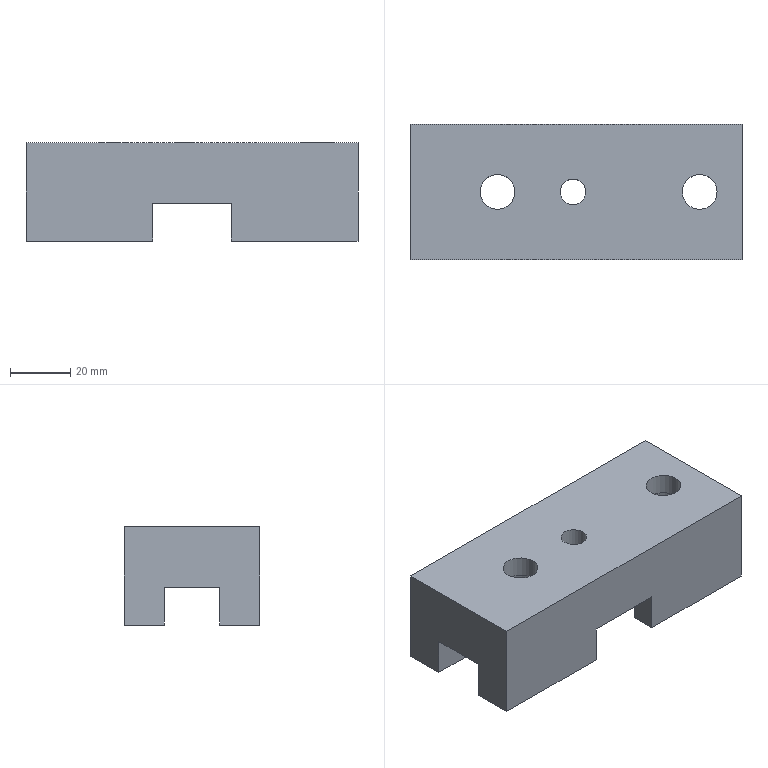Part | STEP file | lll_id3382_x_t | 1 solid | 25 faces | box 110 x 45 x 32.5 mm | volume 112389 mm3 | plane 20 | cylinder 5 | commonest cylinder face diameters 11.509 x2 18.007 x2 8.505 x1
STEP:
#1=CARTESIAN_POINT('',(2756.253,0.00007422,2.5));
#2=VERTEX_POINT('',#1);
#3=CARTESIAN_POINT('',(2752.,0.00007422,2.5));
#4=DIRECTION('',(0.,0.,1.));
#5=DIRECTION('',(1.,0.,0.));
#6=AXIS2_PLACEMENT_3D('',#3,#4,#5);
#7=CIRCLE('',#6,4.253);
#8=EDGE_CURVE('',#2,#2,#7,.T.);
#9=ORIENTED_EDGE('',*,*,#8,.T.);
#10=EDGE_LOOP('',(#9));
#11=FACE_BOUND('',#10,.T.);
#12=CARTESIAN_POINT('',(2766.,-22.5,2.5));
#13=VERTEX_POINT('',#12);
#14=CARTESIAN_POINT('',(2766.,-14.237,2.5));
#15=VERTEX_POINT('',#14);
#16=CARTESIAN_POINT('',(2766.,-9.237,2.5));
#17=DIRECTION('',(0.,1.,0.));
#18=VECTOR('',#17,1.);
#19=LINE('',#16,#18);
#20=EDGE_CURVE('',#13,#15,#19,.T.);
#21=ORIENTED_EDGE('',*,*,#20,.F.);
#22=CARTESIAN_POINT('',(2740.,-22.5,2.5));
#23=VERTEX_POINT('',#22);
#24=CARTESIAN_POINT('',(2733.,-22.5,2.5));
#25=DIRECTION('',(-1.,0.,0.));
#26=VECTOR('',#25,1.);
#27=LINE('',#24,#26);
#28=EDGE_CURVE('',#13,#23,#27,.T.);
#29=ORIENTED_EDGE('',*,*,#28,.T.);
#30=CARTESIAN_POINT('',(2740.,-9.237,2.5));
#31=VERTEX_POINT('',#30);
#32=CARTESIAN_POINT('',(2740.,-26.737,2.5));
#33=DIRECTION('',(0.,-1.,0.));
#34=VECTOR('',#33,1.);
#35=LINE('',#32,#34);
#36=EDGE_CURVE('',#31,#23,#35,.T.);
#37=ORIENTED_EDGE('',*,*,#36,.F.);
#38=CARTESIAN_POINT('',(2698.,-9.237,2.5));
#39=VERTEX_POINT('',#38);
#40=CARTESIAN_POINT('',(2733.,-9.237,2.5));
#41=DIRECTION('',(1.,0.,0.));
#42=VECTOR('',#41,1.);
#43=LINE('',#40,#42);
#44=EDGE_CURVE('',#39,#31,#43,.T.);
#45=ORIENTED_EDGE('',*,*,#44,.F.);
#46=CARTESIAN_POINT('',(2698.,9.237,2.5));
#47=VERTEX_POINT('',#46);
#48=CARTESIAN_POINT('',(2698.,-26.737,2.5));
#49=DIRECTION('',(0.,1.,0.));
#50=VECTOR('',#49,1.);
#51=LINE('',#48,#50);
#52=EDGE_CURVE('',#39,#47,#51,.T.);
#53=ORIENTED_EDGE('',*,*,#52,.T.);
#54=CARTESIAN_POINT('',(2740.,9.237,2.5));
#55=VERTEX_POINT('',#54);
#56=CARTESIAN_POINT('',(2733.,9.237,2.5));
#57=DIRECTION('',(1.,0.,0.));
#58=VECTOR('',#57,1.);
#59=LINE('',#56,#58);
#60=EDGE_CURVE('',#47,#55,#59,.T.);
#61=ORIENTED_EDGE('',*,*,#60,.T.);
#62=CARTESIAN_POINT('',(2740.,22.5,2.5));
#63=VERTEX_POINT('',#62);
#64=CARTESIAN_POINT('',(2740.,26.737,2.5));
#65=DIRECTION('',(0.,1.,0.));
#66=VECTOR('',#65,1.);
#67=LINE('',#64,#66);
#68=EDGE_CURVE('',#55,#63,#67,.T.);
#69=ORIENTED_EDGE('',*,*,#68,.T.);
#70=CARTESIAN_POINT('',(2766.,22.5,2.5));
#71=VERTEX_POINT('',#70);
#72=CARTESIAN_POINT('',(2733.,22.5,2.5));
#73=DIRECTION('',(-1.,0.,0.));
#74=VECTOR('',#73,1.);
#75=LINE('',#72,#74);
#76=EDGE_CURVE('',#71,#63,#75,.T.);
#77=ORIENTED_EDGE('',*,*,#76,.F.);
#78=CARTESIAN_POINT('',(2766.,14.237,2.5));
#79=VERTEX_POINT('',#78);
#80=CARTESIAN_POINT('',(2766.,9.237,2.5));
#81=DIRECTION('',(0.,-1.,0.));
#82=VECTOR('',#81,1.);
#83=LINE('',#80,#82);
#84=EDGE_CURVE('',#71,#79,#83,.T.);
#85=ORIENTED_EDGE('',*,*,#84,.T.);
#86=CARTESIAN_POINT('',(2808.,14.237,2.5));
#87=VERTEX_POINT('',#86);
#88=CARTESIAN_POINT('',(2790.5,14.237,2.5));
#89=DIRECTION('',(-1.,0.,0.));
#90=VECTOR('',#89,1.);
#91=LINE('',#88,#90);
#92=EDGE_CURVE('',#87,#79,#91,.T.);
#93=ORIENTED_EDGE('',*,*,#92,.F.);
#94=CARTESIAN_POINT('',(2808.,-14.237,2.5));
#95=VERTEX_POINT('',#94);
#96=CARTESIAN_POINT('',(2808.,-9.237,2.5));
#97=DIRECTION('',(0.,1.,0.));
#98=VECTOR('',#97,1.);
#99=LINE('',#96,#98);
#100=EDGE_CURVE('',#95,#87,#99,.T.);
#101=ORIENTED_EDGE('',*,*,#100,.F.);
#102=CARTESIAN_POINT('',(2790.5,-14.237,2.5));
#103=DIRECTION('',(-1.,0.,0.));
#104=VECTOR('',#103,1.);
#105=LINE('',#102,#104);
#106=EDGE_CURVE('',#95,#15,#105,.T.);
#107=ORIENTED_EDGE('',*,*,#106,.T.);
#108=EDGE_LOOP('',(#21,#29,#37,#45,#53,#61,#69,#77,#85,#93,#101,#107));
#109=FACE_BOUND('',#108,.T.);
#110=CARTESIAN_POINT('',(2736.003,0.00007422,2.5));
#111=VERTEX_POINT('',#110);
#112=CARTESIAN_POINT('',(2727.,0.00007422,2.5));
#113=DIRECTION('',(0.,0.,1.));
#114=DIRECTION('',(1.,0.,0.));
#115=AXIS2_PLACEMENT_3D('',#112,#113,#114);
#116=CIRCLE('',#115,9.004);
#117=EDGE_CURVE('',#111,#111,#116,.T.);
#118=ORIENTED_EDGE('',*,*,#117,.T.);
#119=EDGE_LOOP('',(#118));
#120=FACE_BOUND('',#119,.T.);
#121=CARTESIAN_POINT('',(2803.004,0.00007422,2.5));
#122=VERTEX_POINT('',#121);
#123=CARTESIAN_POINT('',(2794.,0.00007422,2.5));
#124=DIRECTION('',(0.,0.,1.));
#125=DIRECTION('',(1.,0.,0.));
#126=AXIS2_PLACEMENT_3D('',#123,#124,#125);
#127=CIRCLE('',#126,9.004);
#128=EDGE_CURVE('',#122,#122,#127,.T.);
#129=ORIENTED_EDGE('',*,*,#128,.T.);
#130=EDGE_LOOP('',(#129));
#131=FACE_BOUND('',#130,.T.);
#132=CARTESIAN_POINT('',(2733.,-26.737,2.5));
#133=DIRECTION('',(0.,0.,1.));
#134=DIRECTION('',(1.,0.,0.));
#135=AXIS2_PLACEMENT_3D('',#132,#133,#134);
#136=PLANE('',#135);
#137=ADVANCED_FACE('',(#11,#109,#120,#131),#136,.F.);
#138=CARTESIAN_POINT('',(2747.747,0.00007422,22.5));
#139=VERTEX_POINT('',#138);
#140=CARTESIAN_POINT('',(2752.,0.00007422,22.5));
#141=DIRECTION('',(0.,0.,-1.));
#142=DIRECTION('',(-1.,0.,0.));
#143=AXIS2_PLACEMENT_3D('',#140,#141,#142);
#144=CIRCLE('',#143,4.253);
#145=EDGE_CURVE('',#139,#139,#144,.T.);
#146=ORIENTED_EDGE('',*,*,#145,.T.);
#147=EDGE_LOOP('',(#146));
#148=FACE_BOUND('',#147,.T.);
#149=CARTESIAN_POINT('',(2788.246,0.00007422,22.5));
#150=VERTEX_POINT('',#149);
#151=CARTESIAN_POINT('',(2794.,0.00007422,22.5));
#152=DIRECTION('',(0.,0.,-1.));
#153=DIRECTION('',(-1.,0.,0.));
#154=AXIS2_PLACEMENT_3D('',#151,#152,#153);
#155=CIRCLE('',#154,5.755);
#156=EDGE_CURVE('',#150,#150,#155,.T.);
#157=ORIENTED_EDGE('',*,*,#156,.T.);
#158=EDGE_LOOP('',(#157));
#159=FACE_BOUND('',#158,.T.);
#160=CARTESIAN_POINT('',(2721.245,0.00007422,22.5));
#161=VERTEX_POINT('',#160);
#162=CARTESIAN_POINT('',(2727.,0.00007422,22.5));
#163=DIRECTION('',(0.,0.,-1.));
#164=DIRECTION('',(-1.,0.,0.));
#165=AXIS2_PLACEMENT_3D('',#162,#163,#164);
#166=CIRCLE('',#165,5.755);
#167=EDGE_CURVE('',#161,#161,#166,.T.);
#168=ORIENTED_EDGE('',*,*,#167,.T.);
#169=EDGE_LOOP('',(#168));
#170=FACE_BOUND('',#169,.T.);
#171=CARTESIAN_POINT('',(2698.,22.5,22.5));
#172=VERTEX_POINT('',#171);
#173=CARTESIAN_POINT('',(2698.,-22.5,22.5));
#174=VERTEX_POINT('',#173);
#175=CARTESIAN_POINT('',(2698.,40.,22.5));
#176=DIRECTION('',(0.,-1.,0.));
#177=VECTOR('',#176,1.);
#178=LINE('',#175,#177);
#179=EDGE_CURVE('',#172,#174,#178,.T.);
#180=ORIENTED_EDGE('',*,*,#179,.T.);
#181=CARTESIAN_POINT('',(2808.,-22.5,22.5));
#182=VERTEX_POINT('',#181);
#183=CARTESIAN_POINT('',(2733.,-22.5,22.5));
#184=DIRECTION('',(-1.,0.,0.));
#185=VECTOR('',#184,1.);
#186=LINE('',#183,#185);
#187=EDGE_CURVE('',#182,#174,#186,.T.);
#188=ORIENTED_EDGE('',*,*,#187,.F.);
#189=CARTESIAN_POINT('',(2808.,22.5,22.5));
#190=VERTEX_POINT('',#189);
#191=CARTESIAN_POINT('',(2808.,26.737,22.5));
#192=DIRECTION('',(0.,-1.,0.));
#193=VECTOR('',#192,1.);
#194=LINE('',#191,#193);
#195=EDGE_CURVE('',#190,#182,#194,.T.);
#196=ORIENTED_EDGE('',*,*,#195,.F.);
#197=CARTESIAN_POINT('',(2733.,22.5,22.5));
#198=DIRECTION('',(-1.,0.,0.));
#199=VECTOR('',#198,1.);
#200=LINE('',#197,#199);
#201=EDGE_CURVE('',#190,#172,#200,.T.);
#202=ORIENTED_EDGE('',*,*,#201,.T.);
#203=EDGE_LOOP('',(#180,#188,#196,#202));
#204=FACE_BOUND('',#203,.T.);
#205=CARTESIAN_POINT('',(2733.,40.,22.5));
#206=DIRECTION('',(0.,0.,-1.));
#207=DIRECTION('',(-1.,0.,0.));
#208=AXIS2_PLACEMENT_3D('',#205,#206,#207);
#209=PLANE('',#208);
#210=ADVANCED_FACE('',(#148,#159,#170,#204),#209,.F.);
#211=CARTESIAN_POINT('',(2698.,-22.5,-10.));
#212=VERTEX_POINT('',#211);
#213=CARTESIAN_POINT('',(2698.,-9.237,-10.));
#214=VERTEX_POINT('',#213);
#215=CARTESIAN_POINT('',(2698.,1.,-10.));
#216=DIRECTION('',(0.,1.,0.));
#217=VECTOR('',#216,1.);
#218=LINE('',#215,#217);
#219=EDGE_CURVE('',#212,#214,#218,.T.);
#220=ORIENTED_EDGE('',*,*,#219,.F.);
#221=CARTESIAN_POINT('',(2698.,-22.5,12.5));
#222=DIRECTION('',(0.,0.,-1.));
#223=VECTOR('',#222,1.);
#224=LINE('',#221,#223);
#225=EDGE_CURVE('',#174,#212,#224,.T.);
#226=ORIENTED_EDGE('',*,*,#225,.F.);
#227=ORIENTED_EDGE('',*,*,#179,.F.);
#228=CARTESIAN_POINT('',(2698.,22.5,-10.));
#229=VERTEX_POINT('',#228);
#230=CARTESIAN_POINT('',(2698.,22.5,12.5));
#231=DIRECTION('',(0.,0.,-1.));
#232=VECTOR('',#231,1.);
#233=LINE('',#230,#232);
#234=EDGE_CURVE('',#172,#229,#233,.T.);
#235=ORIENTED_EDGE('',*,*,#234,.T.);
#236=CARTESIAN_POINT('',(2698.,9.237,-10.));
#237=VERTEX_POINT('',#236);
#238=CARTESIAN_POINT('',(2698.,-0.9999,-10.));
#239=DIRECTION('',(0.,-1.,0.));
#240=VECTOR('',#239,1.);
#241=LINE('',#238,#240);
#242=EDGE_CURVE('',#229,#237,#241,.T.);
#243=ORIENTED_EDGE('',*,*,#242,.T.);
#244=CARTESIAN_POINT('',(2698.,9.237,-2.5));
#245=DIRECTION('',(0.,0.,1.));
#246=VECTOR('',#245,1.);
#247=LINE('',#244,#246);
#248=EDGE_CURVE('',#237,#47,#247,.T.);
#249=ORIENTED_EDGE('',*,*,#248,.T.);
#250=ORIENTED_EDGE('',*,*,#52,.F.);
#251=CARTESIAN_POINT('',(2698.,-9.237,-2.5));
#252=DIRECTION('',(0.,0.,1.));
#253=VECTOR('',#252,1.);
#254=LINE('',#251,#253);
#255=EDGE_CURVE('',#214,#39,#254,.T.);
#256=ORIENTED_EDGE('',*,*,#255,.F.);
#257=EDGE_LOOP('',(#220,#226,#227,#235,#243,#249,#250,#256));
#258=FACE_OUTER_BOUND('',#257,.T.);
#259=CARTESIAN_POINT('',(2698.,-26.737,12.5));
#260=DIRECTION('',(1.,0.,0.));
#261=DIRECTION('',(0.,0.,-1.));
#262=AXIS2_PLACEMENT_3D('',#259,#260,#261);
#263=PLANE('',#262);
#264=ADVANCED_FACE('',(#258),#263,.F.);
#265=ORIENTED_EDGE('',*,*,#195,.T.);
#266=CARTESIAN_POINT('',(2808.,-22.5,-10.));
#267=VERTEX_POINT('',#266);
#268=CARTESIAN_POINT('',(2808.,-22.5,12.5));
#269=DIRECTION('',(0.,0.,-1.));
#270=VECTOR('',#269,1.);
#271=LINE('',#268,#270);
#272=EDGE_CURVE('',#182,#267,#271,.T.);
#273=ORIENTED_EDGE('',*,*,#272,.T.);
#274=CARTESIAN_POINT('',(2808.,-14.237,-10.));
#275=VERTEX_POINT('',#274);
#276=CARTESIAN_POINT('',(2808.,1.,-10.));
#277=DIRECTION('',(0.,1.,0.));
#278=VECTOR('',#277,1.);
#279=LINE('',#276,#278);
#280=EDGE_CURVE('',#267,#275,#279,.T.);
#281=ORIENTED_EDGE('',*,*,#280,.T.);
#282=CARTESIAN_POINT('',(2808.,-14.237,12.5));
#283=DIRECTION('',(0.,0.,1.));
#284=VECTOR('',#283,1.);
#285=LINE('',#282,#284);
#286=EDGE_CURVE('',#275,#95,#285,.T.);
#287=ORIENTED_EDGE('',*,*,#286,.T.);
#288=ORIENTED_EDGE('',*,*,#100,.T.);
#289=CARTESIAN_POINT('',(2808.,14.237,-10.));
#290=VERTEX_POINT('',#289);
#291=CARTESIAN_POINT('',(2808.,14.237,12.5));
#292=DIRECTION('',(0.,0.,1.));
#293=VECTOR('',#292,1.);
#294=LINE('',#291,#293);
#295=EDGE_CURVE('',#290,#87,#294,.T.);
#296=ORIENTED_EDGE('',*,*,#295,.F.);
#297=CARTESIAN_POINT('',(2808.,22.5,-10.));
#298=VERTEX_POINT('',#297);
#299=CARTESIAN_POINT('',(2808.,-0.9999,-10.));
#300=DIRECTION('',(0.,-1.,0.));
#301=VECTOR('',#300,1.);
#302=LINE('',#299,#301);
#303=EDGE_CURVE('',#298,#290,#302,.T.);
#304=ORIENTED_EDGE('',*,*,#303,.F.);
#305=CARTESIAN_POINT('',(2808.,22.5,12.5));
#306=DIRECTION('',(0.,0.,-1.));
#307=VECTOR('',#306,1.);
#308=LINE('',#305,#307);
#309=EDGE_CURVE('',#190,#298,#308,.T.);
#310=ORIENTED_EDGE('',*,*,#309,.F.);
#311=EDGE_LOOP('',(#265,#273,#281,#287,#288,#296,#304,#310));
#312=FACE_OUTER_BOUND('',#311,.T.);
#313=CARTESIAN_POINT('',(2808.,-26.737,12.5));
#314=DIRECTION('',(-1.,0.,0.));
#315=DIRECTION('',(0.,0.,-1.));
#316=AXIS2_PLACEMENT_3D('',#313,#314,#315);
#317=PLANE('',#316);
#318=ADVANCED_FACE('',(#312),#317,.F.);
#319=ORIENTED_EDGE('',*,*,#36,.T.);
#320=CARTESIAN_POINT('',(2740.,-22.5,-10.));
#321=VERTEX_POINT('',#320);
#322=CARTESIAN_POINT('',(2740.,-22.5,12.5));
#323=DIRECTION('',(0.,0.,-1.));
#324=VECTOR('',#323,1.);
#325=LINE('',#322,#324);
#326=EDGE_CURVE('',#23,#321,#325,.T.);
#327=ORIENTED_EDGE('',*,*,#326,.T.);
#328=CARTESIAN_POINT('',(2740.,-9.237,-10.));
#329=VERTEX_POINT('',#328);
#330=CARTESIAN_POINT('',(2740.,1.,-10.));
#331=DIRECTION('',(0.,1.,0.));
#332=VECTOR('',#331,1.);
#333=LINE('',#330,#332);
#334=EDGE_CURVE('',#321,#329,#333,.T.);
#335=ORIENTED_EDGE('',*,*,#334,.T.);
#336=CARTESIAN_POINT('',(2740.,-9.237,-2.5));
#337=DIRECTION('',(0.,0.,1.));
#338=VECTOR('',#337,1.);
#339=LINE('',#336,#338);
#340=EDGE_CURVE('',#329,#31,#339,.T.);
#341=ORIENTED_EDGE('',*,*,#340,.T.);
#342=EDGE_LOOP('',(#319,#327,#335,#341));
#343=FACE_OUTER_BOUND('',#342,.T.);
#344=CARTESIAN_POINT('',(2740.,-26.737,12.5));
#345=DIRECTION('',(1.,0.,0.));
#346=DIRECTION('',(0.,0.,-1.));
#347=AXIS2_PLACEMENT_3D('',#344,#345,#346);
#348=PLANE('',#347);
#349=ADVANCED_FACE('',(#343),#348,.T.);
#350=ORIENTED_EDGE('',*,*,#334,.F.);
#351=CARTESIAN_POINT('',(6303.751,-22.5,-10.));
#352=DIRECTION('',(1.,0.,0.));
#353=VECTOR('',#352,1.);
#354=LINE('',#351,#353);
#355=EDGE_CURVE('',#212,#321,#354,.T.);
#356=ORIENTED_EDGE('',*,*,#355,.F.);
#357=ORIENTED_EDGE('',*,*,#219,.T.);
#358=CARTESIAN_POINT('',(2715.5,-9.237,-10.));
#359=DIRECTION('',(-1.,0.,0.));
#360=VECTOR('',#359,1.);
#361=LINE('',#358,#360);
#362=EDGE_CURVE('',#329,#214,#361,.T.);
#363=ORIENTED_EDGE('',*,*,#362,.F.);
#364=EDGE_LOOP('',(#350,#356,#357,#363));
#365=FACE_OUTER_BOUND('',#364,.T.);
#366=CARTESIAN_POINT('',(6303.751,1.,-10.));
#367=DIRECTION('',(0.,0.,1.));
#368=DIRECTION('',(1.,0.,0.));
#369=AXIS2_PLACEMENT_3D('',#366,#367,#368);
#370=PLANE('',#369);
#371=ADVANCED_FACE('',(#365),#370,.F.);
#372=ORIENTED_EDGE('',*,*,#362,.T.);
#373=ORIENTED_EDGE('',*,*,#255,.T.);
#374=ORIENTED_EDGE('',*,*,#44,.T.);
#375=ORIENTED_EDGE('',*,*,#340,.F.);
#376=EDGE_LOOP('',(#372,#373,#374,#375));
#377=FACE_OUTER_BOUND('',#376,.T.);
#378=CARTESIAN_POINT('',(2715.5,-9.237,-2.5));
#379=DIRECTION('',(0.,-1.,0.));
#380=DIRECTION('',(0.,0.,-1.));
#381=AXIS2_PLACEMENT_3D('',#378,#379,#380);
#382=PLANE('',#381);
#383=ADVANCED_FACE('',(#377),#382,.F.);
#384=ORIENTED_EDGE('',*,*,#280,.F.);
#385=CARTESIAN_POINT('',(2766.,-22.5,-10.));
#386=VERTEX_POINT('',#385);
#387=CARTESIAN_POINT('',(-797.751,-22.5,-10.));
#388=DIRECTION('',(-1.,0.,0.));
#389=VECTOR('',#388,1.);
#390=LINE('',#387,#389);
#391=EDGE_CURVE('',#267,#386,#390,.T.);
#392=ORIENTED_EDGE('',*,*,#391,.T.);
#393=CARTESIAN_POINT('',(2766.,-14.237,-10.));
#394=VERTEX_POINT('',#393);
#395=CARTESIAN_POINT('',(2766.,1.,-10.));
#396=DIRECTION('',(0.,1.,0.));
#397=VECTOR('',#396,1.);
#398=LINE('',#395,#397);
#399=EDGE_CURVE('',#386,#394,#398,.T.);
#400=ORIENTED_EDGE('',*,*,#399,.T.);
#401=CARTESIAN_POINT('',(-797.751,-14.237,-10.));
#402=DIRECTION('',(1.,0.,0.));
#403=VECTOR('',#402,1.);
#404=LINE('',#401,#403);
#405=EDGE_CURVE('',#394,#275,#404,.T.);
#406=ORIENTED_EDGE('',*,*,#405,.T.);
#407=EDGE_LOOP('',(#384,#392,#400,#406));
#408=FACE_OUTER_BOUND('',#407,.T.);
#409=CARTESIAN_POINT('',(-797.751,1.,-10.));
#410=DIRECTION('',(0.,0.,1.));
#411=DIRECTION('',(-1.,0.,0.));
#412=AXIS2_PLACEMENT_3D('',#409,#410,#411);
#413=PLANE('',#412);
#414=ADVANCED_FACE('',(#408),#413,.F.);
#415=ORIENTED_EDGE('',*,*,#399,.F.);
#416=CARTESIAN_POINT('',(2766.,-22.5,12.5));
#417=DIRECTION('',(0.,0.,-1.));
#418=VECTOR('',#417,1.);
#419=LINE('',#416,#418);
#420=EDGE_CURVE('',#13,#386,#419,.T.);
#421=ORIENTED_EDGE('',*,*,#420,.F.);
#422=ORIENTED_EDGE('',*,*,#20,.T.);
#423=CARTESIAN_POINT('',(2766.,-14.237,12.5));
#424=DIRECTION('',(0.,0.,1.));
#425=VECTOR('',#424,1.);
#426=LINE('',#423,#425);
#427=EDGE_CURVE('',#394,#15,#426,.T.);
#428=ORIENTED_EDGE('',*,*,#427,.F.);
#429=EDGE_LOOP('',(#415,#421,#422,#428));
#430=FACE_OUTER_BOUND('',#429,.T.);
#431=CARTESIAN_POINT('',(2766.,-26.737,12.5));
#432=DIRECTION('',(-1.,0.,0.));
#433=DIRECTION('',(0.,0.,-1.));
#434=AXIS2_PLACEMENT_3D('',#431,#432,#433);
#435=PLANE('',#434);
#436=ADVANCED_FACE('',(#430),#435,.T.);
#437=ORIENTED_EDGE('',*,*,#405,.F.);
#438=ORIENTED_EDGE('',*,*,#427,.T.);
#439=ORIENTED_EDGE('',*,*,#106,.F.);
#440=ORIENTED_EDGE('',*,*,#286,.F.);
#441=EDGE_LOOP('',(#437,#438,#439,#440));
#442=FACE_OUTER_BOUND('',#441,.T.);
#443=CARTESIAN_POINT('',(2790.5,-14.237,-2.5));
#444=DIRECTION('',(0.,-1.,0.));
#445=DIRECTION('',(0.,0.,-1.));
#446=AXIS2_PLACEMENT_3D('',#443,#444,#445);
#447=PLANE('',#446);
#448=ADVANCED_FACE('',(#442),#447,.F.);
#449=ORIENTED_EDGE('',*,*,#28,.F.);
#450=ORIENTED_EDGE('',*,*,#420,.T.);
#451=ORIENTED_EDGE('',*,*,#391,.F.);
#452=ORIENTED_EDGE('',*,*,#272,.F.);
#453=ORIENTED_EDGE('',*,*,#187,.T.);
#454=ORIENTED_EDGE('',*,*,#225,.T.);
#455=ORIENTED_EDGE('',*,*,#355,.T.);
#456=ORIENTED_EDGE('',*,*,#326,.F.);
#457=EDGE_LOOP('',(#449,#450,#451,#452,#453,#454,#455,#456));
#458=FACE_OUTER_BOUND('',#457,.T.);
#459=CARTESIAN_POINT('',(2753.,-22.5,12.5));
#460=DIRECTION('',(0.,1.,0.));
#461=DIRECTION('',(0.,0.,1.));
#462=AXIS2_PLACEMENT_3D('',#459,#460,#461);
#463=PLANE('',#462);
#464=ADVANCED_FACE('',(#458),#463,.F.);
#465=ORIENTED_EDGE('',*,*,#68,.F.);
#466=CARTESIAN_POINT('',(2740.,9.237,-10.));
#467=VERTEX_POINT('',#466);
#468=CARTESIAN_POINT('',(2740.,9.237,-2.5));
#469=DIRECTION('',(0.,0.,1.));
#470=VECTOR('',#469,1.);
#471=LINE('',#468,#470);
#472=EDGE_CURVE('',#467,#55,#471,.T.);
#473=ORIENTED_EDGE('',*,*,#472,.F.);
#474=CARTESIAN_POINT('',(2740.,22.5,-10.));
#475=VERTEX_POINT('',#474);
#476=CARTESIAN_POINT('',(2740.,-0.9999,-10.));
#477=DIRECTION('',(0.,-1.,0.));
#478=VECTOR('',#477,1.);
#479=LINE('',#476,#478);
#480=EDGE_CURVE('',#475,#467,#479,.T.);
#481=ORIENTED_EDGE('',*,*,#480,.F.);
#482=CARTESIAN_POINT('',(2740.,22.5,12.5));
#483=DIRECTION('',(0.,0.,-1.));
#484=VECTOR('',#483,1.);
#485=LINE('',#482,#484);
#486=EDGE_CURVE('',#63,#475,#485,.T.);
#487=ORIENTED_EDGE('',*,*,#486,.F.);
#488=EDGE_LOOP('',(#465,#473,#481,#487));
#489=FACE_OUTER_BOUND('',#488,.T.);
#490=CARTESIAN_POINT('',(2740.,26.737,12.5));
#491=DIRECTION('',(1.,0.,0.));
#492=DIRECTION('',(0.,0.,-1.));
#493=AXIS2_PLACEMENT_3D('',#490,#491,#492);
#494=PLANE('',#493);
#495=ADVANCED_FACE('',(#489),#494,.T.);
#496=CARTESIAN_POINT('',(6303.751,22.5,-10.));
#497=DIRECTION('',(1.,0.,0.));
#498=VECTOR('',#497,1.);
#499=LINE('',#496,#498);
#500=EDGE_CURVE('',#229,#475,#499,.T.);
#501=ORIENTED_EDGE('',*,*,#500,.T.);
#502=ORIENTED_EDGE('',*,*,#480,.T.);
#503=CARTESIAN_POINT('',(2715.5,9.237,-10.));
#504=DIRECTION('',(-1.,0.,0.));
#505=VECTOR('',#504,1.);
#506=LINE('',#503,#505);
#507=EDGE_CURVE('',#467,#237,#506,.T.);
#508=ORIENTED_EDGE('',*,*,#507,.T.);
#509=ORIENTED_EDGE('',*,*,#242,.F.);
#510=EDGE_LOOP('',(#501,#502,#508,#509));
#511=FACE_OUTER_BOUND('',#510,.T.);
#512=CARTESIAN_POINT('',(6303.751,-0.9999,-10.));
#513=DIRECTION('',(0.,0.,1.));
#514=DIRECTION('',(1.,0.,0.));
#515=AXIS2_PLACEMENT_3D('',#512,#513,#514);
#516=PLANE('',#515);
#517=ADVANCED_FACE('',(#511),#516,.F.);
#518=ORIENTED_EDGE('',*,*,#507,.F.);
#519=ORIENTED_EDGE('',*,*,#472,.T.);
#520=ORIENTED_EDGE('',*,*,#60,.F.);
#521=ORIENTED_EDGE('',*,*,#248,.F.);
#522=EDGE_LOOP('',(#518,#519,#520,#521));
#523=FACE_OUTER_BOUND('',#522,.T.);
#524=CARTESIAN_POINT('',(2715.5,9.237,-2.5));
#525=DIRECTION('',(0.,1.,0.));
#526=DIRECTION('',(0.,0.,-1.));
#527=AXIS2_PLACEMENT_3D('',#524,#525,#526);
#528=PLANE('',#527);
#529=ADVANCED_FACE('',(#523),#528,.F.);
#530=ORIENTED_EDGE('',*,*,#303,.T.);
#531=CARTESIAN_POINT('',(2766.,14.237,-10.));
#532=VERTEX_POINT('',#531);
#533=CARTESIAN_POINT('',(-797.751,14.237,-10.));
#534=DIRECTION('',(1.,0.,0.));
#535=VECTOR('',#534,1.);
#536=LINE('',#533,#535);
#537=EDGE_CURVE('',#532,#290,#536,.T.);
#538=ORIENTED_EDGE('',*,*,#537,.F.);
#539=CARTESIAN_POINT('',(2766.,22.5,-10.));
#540=VERTEX_POINT('',#539);
#541=CARTESIAN_POINT('',(2766.,-0.9999,-10.));
#542=DIRECTION('',(0.,-1.,0.));
#543=VECTOR('',#542,1.);
#544=LINE('',#541,#543);
#545=EDGE_CURVE('',#540,#532,#544,.T.);
#546=ORIENTED_EDGE('',*,*,#545,.F.);
#547=CARTESIAN_POINT('',(-797.751,22.5,-10.));
#548=DIRECTION('',(-1.,0.,0.));
#549=VECTOR('',#548,1.);
#550=LINE('',#547,#549);
#551=EDGE_CURVE('',#298,#540,#550,.T.);
#552=ORIENTED_EDGE('',*,*,#551,.F.);
#553=EDGE_LOOP('',(#530,#538,#546,#552));
#554=FACE_OUTER_BOUND('',#553,.T.);
#555=CARTESIAN_POINT('',(-797.751,-0.9999,-10.));
#556=DIRECTION('',(0.,0.,1.));
#557=DIRECTION('',(-1.,0.,0.));
#558=AXIS2_PLACEMENT_3D('',#555,#556,#557);
#559=PLANE('',#558);
#560=ADVANCED_FACE('',(#554),#559,.F.);
#561=ORIENTED_EDGE('',*,*,#84,.F.);
#562=CARTESIAN_POINT('',(2766.,22.5,12.5));
#563=DIRECTION('',(0.,0.,-1.));
#564=VECTOR('',#563,1.);
#565=LINE('',#562,#564);
#566=EDGE_CURVE('',#71,#540,#565,.T.);
#567=ORIENTED_EDGE('',*,*,#566,.T.);
#568=ORIENTED_EDGE('',*,*,#545,.T.);
#569=CARTESIAN_POINT('',(2766.,14.237,12.5));
#570=DIRECTION('',(0.,0.,1.));
#571=VECTOR('',#570,1.);
#572=LINE('',#569,#571);
#573=EDGE_CURVE('',#532,#79,#572,.T.);
#574=ORIENTED_EDGE('',*,*,#573,.T.);
#575=EDGE_LOOP('',(#561,#567,#568,#574));
#576=FACE_OUTER_BOUND('',#575,.T.);
#577=CARTESIAN_POINT('',(2766.,26.737,12.5));
#578=DIRECTION('',(-1.,0.,0.));
#579=DIRECTION('',(0.,0.,-1.));
#580=AXIS2_PLACEMENT_3D('',#577,#578,#579);
#581=PLANE('',#580);
#582=ADVANCED_FACE('',(#576),#581,.T.);
#583=ORIENTED_EDGE('',*,*,#537,.T.);
#584=ORIENTED_EDGE('',*,*,#295,.T.);
#585=ORIENTED_EDGE('',*,*,#92,.T.);
#586=ORIENTED_EDGE('',*,*,#573,.F.);
#587=EDGE_LOOP('',(#583,#584,#585,#586));
#588=FACE_OUTER_BOUND('',#587,.T.);
#589=CARTESIAN_POINT('',(2790.5,14.237,-2.5));
#590=DIRECTION('',(0.,1.,0.));
#591=DIRECTION('',(0.,0.,-1.));
#592=AXIS2_PLACEMENT_3D('',#589,#590,#591);
#593=PLANE('',#592);
#594=ADVANCED_FACE('',(#588),#593,.F.);
#595=ORIENTED_EDGE('',*,*,#566,.F.);
#596=ORIENTED_EDGE('',*,*,#76,.T.);
#597=ORIENTED_EDGE('',*,*,#486,.T.);
#598=ORIENTED_EDGE('',*,*,#500,.F.);
#599=ORIENTED_EDGE('',*,*,#234,.F.);
#600=ORIENTED_EDGE('',*,*,#201,.F.);
#601=ORIENTED_EDGE('',*,*,#309,.T.);
#602=ORIENTED_EDGE('',*,*,#551,.T.);
#603=EDGE_LOOP('',(#595,#596,#597,#598,#599,#600,#601,#602));
#604=FACE_OUTER_BOUND('',#603,.T.);
#605=CARTESIAN_POINT('',(2753.,22.5,12.5));
#606=DIRECTION('',(0.,-1.,0.));
#607=DIRECTION('',(0.,0.,1.));
#608=AXIS2_PLACEMENT_3D('',#605,#606,#607);
#609=PLANE('',#608);
#610=ADVANCED_FACE('',(#604),#609,.F.);
#611=CARTESIAN_POINT('',(2732.755,0.00007422,15.5));
#612=VERTEX_POINT('',#611);
#613=CARTESIAN_POINT('',(2727.,0.00007422,15.5));
#614=DIRECTION('',(0.,0.,1.));
#615=DIRECTION('',(1.,0.,0.));
#616=AXIS2_PLACEMENT_3D('',#613,#614,#615);
#617=CIRCLE('',#616,5.755);
#618=EDGE_CURVE('',#612,#612,#617,.T.);
#619=ORIENTED_EDGE('',*,*,#618,.F.);
#620=EDGE_LOOP('',(#619));
#621=FACE_BOUND('',#620,.T.);
#622=ORIENTED_EDGE('',*,*,#167,.F.);
#623=EDGE_LOOP('',(#622));
#624=FACE_BOUND('',#623,.T.);
#625=CARTESIAN_POINT('',(2727.,0.00007422,-2.5));
#626=DIRECTION('',(0.,0.,1.));
#627=DIRECTION('',(1.,0.,0.));
#628=AXIS2_PLACEMENT_3D('',#625,#626,#627);
#629=CYLINDRICAL_SURFACE('',#628,5.755);
#630=ADVANCED_FACE('',(#621,#624),#629,.F.);
#631=ORIENTED_EDGE('',*,*,#618,.T.);
#632=EDGE_LOOP('',(#631));
#633=FACE_BOUND('',#632,.T.);
#634=CARTESIAN_POINT('',(2736.003,0.00007422,15.5));
#635=VERTEX_POINT('',#634);
#636=CARTESIAN_POINT('',(2727.,0.00007422,15.5));
#637=DIRECTION('',(0.,0.,1.));
#638=DIRECTION('',(1.,0.,0.));
#639=AXIS2_PLACEMENT_3D('',#636,#637,#638);
#640=CIRCLE('',#639,9.004);
#641=EDGE_CURVE('',#635,#635,#640,.T.);
#642=ORIENTED_EDGE('',*,*,#641,.F.);
#643=EDGE_LOOP('',(#642));
#644=FACE_BOUND('',#643,.T.);
#645=CARTESIAN_POINT('',(2727.,0.00007422,15.5));
#646=DIRECTION('',(0.,0.,1.));
#647=DIRECTION('',(1.,0.,0.));
#648=AXIS2_PLACEMENT_3D('',#645,#646,#647);
#649=PLANE('',#648);
#650=ADVANCED_FACE('',(#633,#644),#649,.F.);
#651=ORIENTED_EDGE('',*,*,#641,.T.);
#652=EDGE_LOOP('',(#651));
#653=FACE_BOUND('',#652,.T.);
#654=ORIENTED_EDGE('',*,*,#117,.F.);
#655=EDGE_LOOP('',(#654));
#656=FACE_BOUND('',#655,.T.);
#657=CARTESIAN_POINT('',(2727.,0.00007422,2.5));
#658=DIRECTION('',(0.,0.,1.));
#659=DIRECTION('',(1.,0.,0.));
#660=AXIS2_PLACEMENT_3D('',#657,#658,#659);
#661=CYLINDRICAL_SURFACE('',#660,9.004);
#662=ADVANCED_FACE('',(#653,#656),#661,.F.);
#663=CARTESIAN_POINT('',(2799.755,0.00007422,15.5));
#664=VERTEX_POINT('',#663);
#665=CARTESIAN_POINT('',(2794.,0.00007422,15.5));
#666=DIRECTION('',(0.,0.,1.));
#667=DIRECTION('',(1.,0.,0.));
#668=AXIS2_PLACEMENT_3D('',#665,#666,#667);
#669=CIRCLE('',#668,5.755);
#670=EDGE_CURVE('',#664,#664,#669,.T.);
#671=ORIENTED_EDGE('',*,*,#670,.F.);
#672=EDGE_LOOP('',(#671));
#673=FACE_BOUND('',#672,.T.);
#674=ORIENTED_EDGE('',*,*,#156,.F.);
#675=EDGE_LOOP('',(#674));
#676=FACE_BOUND('',#675,.T.);
#677=CARTESIAN_POINT('',(2794.,0.00007422,-2.5));
#678=DIRECTION('',(0.,0.,1.));
#679=DIRECTION('',(1.,0.,0.));
#680=AXIS2_PLACEMENT_3D('',#677,#678,#679);
#681=CYLINDRICAL_SURFACE('',#680,5.755);
#682=ADVANCED_FACE('',(#673,#676),#681,.F.);
#683=ORIENTED_EDGE('',*,*,#670,.T.);
#684=EDGE_LOOP('',(#683));
#685=FACE_BOUND('',#684,.T.);
#686=CARTESIAN_POINT('',(2803.004,0.00007422,15.5));
#687=VERTEX_POINT('',#686);
#688=CARTESIAN_POINT('',(2794.,0.00007422,15.5));
#689=DIRECTION('',(0.,0.,1.));
#690=DIRECTION('',(1.,0.,0.));
#691=AXIS2_PLACEMENT_3D('',#688,#689,#690);
#692=CIRCLE('',#691,9.004);
#693=EDGE_CURVE('',#687,#687,#692,.T.);
#694=ORIENTED_EDGE('',*,*,#693,.F.);
#695=EDGE_LOOP('',(#694));
#696=FACE_BOUND('',#695,.T.);
#697=CARTESIAN_POINT('',(2794.,0.00007422,15.5));
#698=DIRECTION('',(0.,0.,1.));
#699=DIRECTION('',(1.,0.,0.));
#700=AXIS2_PLACEMENT_3D('',#697,#698,#699);
#701=PLANE('',#700);
#702=ADVANCED_FACE('',(#685,#696),#701,.F.);
#703=ORIENTED_EDGE('',*,*,#693,.T.);
#704=EDGE_LOOP('',(#703));
#705=FACE_BOUND('',#704,.T.);
#706=ORIENTED_EDGE('',*,*,#128,.F.);
#707=EDGE_LOOP('',(#706));
#708=FACE_BOUND('',#707,.T.);
#709=CARTESIAN_POINT('',(2794.,0.00007422,2.5));
#710=DIRECTION('',(0.,0.,1.));
#711=DIRECTION('',(1.,0.,0.));
#712=AXIS2_PLACEMENT_3D('',#709,#710,#711);
#713=CYLINDRICAL_SURFACE('',#712,9.004);
#714=ADVANCED_FACE('',(#705,#708),#713,.F.);
#715=ORIENTED_EDGE('',*,*,#8,.F.);
#716=EDGE_LOOP('',(#715));
#717=FACE_BOUND('',#716,.T.);
#718=ORIENTED_EDGE('',*,*,#145,.F.);
#719=EDGE_LOOP('',(#718));
#720=FACE_BOUND('',#719,.T.);
#721=CARTESIAN_POINT('',(2752.,0.00007422,2.5));
#722=DIRECTION('',(0.,0.,1.));
#723=DIRECTION('',(1.,0.,0.));
#724=AXIS2_PLACEMENT_3D('',#721,#722,#723);
#725=CYLINDRICAL_SURFACE('',#724,4.253);
#726=ADVANCED_FACE('',(#717,#720),#725,.F.);
#727=CLOSED_SHELL('',(#137,#210,#264,#318,#349,#371,#383,#414,#436,#448,#464,#495,#517,#529,#560,#582,#594,#610,#630,#650,#662,#682,#702,#714,#726));
#728=MANIFOLD_SOLID_BREP('',#727);
#729=(LENGTH_UNIT()NAMED_UNIT(*)SI_UNIT(.MILLI.,.METRE.));
#730=UNCERTAINTY_MEASURE_WITH_UNIT(LENGTH_MEASURE(0.00002),#729,'','');
#731=(NAMED_UNIT(*)PLANE_ANGLE_UNIT()SI_UNIT($,.RADIAN.));
#732=PLANE_ANGLE_MEASURE_WITH_UNIT(PLANE_ANGLE_MEASURE(0.01745),#731);
#733=DIMENSIONAL_EXPONENTS(0.,0.,0.,0.,0.,0.,0.);
#734=(CONVERSION_BASED_UNIT('DEGREE',#732)NAMED_UNIT(#733)PLANE_ANGLE_UNIT());
#735=(NAMED_UNIT(*)SI_UNIT($,.STERADIAN.)SOLID_ANGLE_UNIT());
#736=(GEOMETRIC_REPRESENTATION_CONTEXT(3)GLOBAL_UNCERTAINTY_ASSIGNED_CONTEXT((#730))GLOBAL_UNIT_ASSIGNED_CONTEXT((#729,#734,#735))REPRESENTATION_CONTEXT('',''));
#737=ADVANCED_BREP_SHAPE_REPRESENTATION('',(#728),#736);